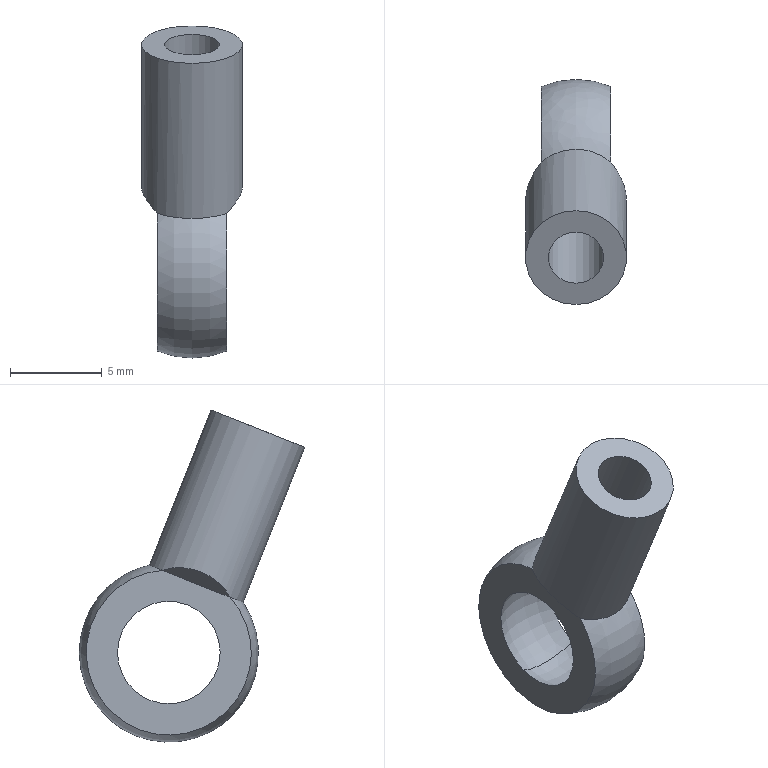Part | STEP file | _.0mm Dowel Hole1 | 1 solid | 11 faces | box 5.5 x 12.284 x 18.097 mm | volume 294.625 mm3 | plane 5 | spline 3 | cylinder 2 | cone 1 | commonest cylinder face diameters 3 x1 5.5 x1